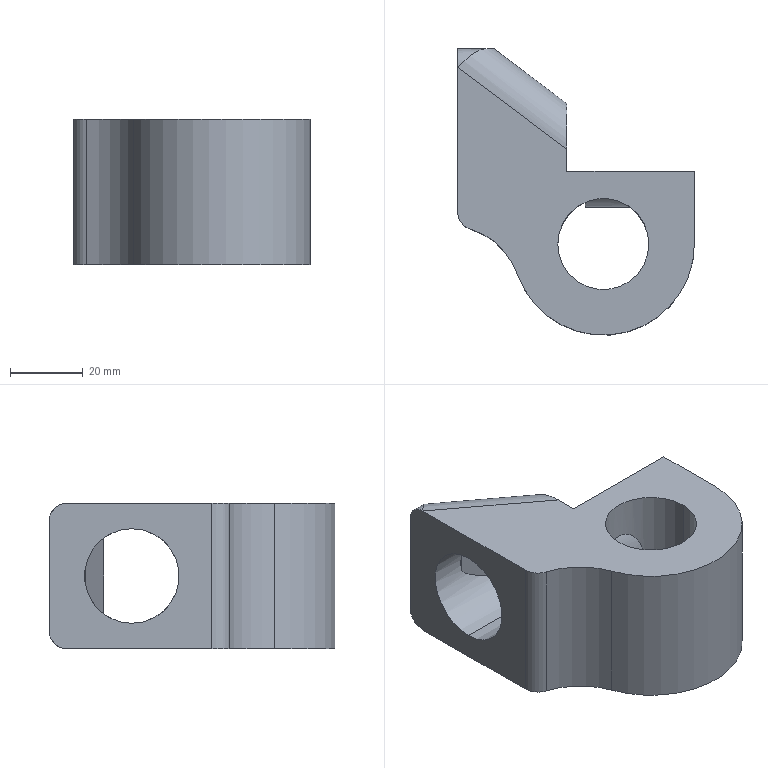Part | SolidWorks | features Cut 5, Fillet 4, ICE 4, Extrusion 1 | 1 solid | 29 faces | box 65 x 78.563 x 40 mm | volume 84441 mm3 | plane 15 | cylinder 14 | commonest cylinder face diameters 10 x3 41.45 x3 20 x2 25 x2 26 x2 40 x1
STEP:
#1=CARTESIAN_POINT('',(82.5,25.,40.));
#2=VERTEX_POINT('',#1);
#3=CARTESIAN_POINT('',(57.5,25.,40.));
#4=VERTEX_POINT('',#3);
#5=CARTESIAN_POINT('',(70.,25.,40.));
#6=DIRECTION('',(0.,0.,-1.));
#7=DIRECTION('',(-1.,0.,0.));
#8=AXIS2_PLACEMENT_3D('',#5,#6,#7);
#9=CIRCLE('',#8,12.5);
#10=EDGE_CURVE('',#2,#4,#9,.T.);
#11=ORIENTED_EDGE('',*,*,#10,.F.);
#12=CARTESIAN_POINT('',(82.5,25.,0.));
#13=VERTEX_POINT('',#12);
#14=CARTESIAN_POINT('',(82.5,25.,40.));
#15=DIRECTION('',(0.,0.,-1.));
#16=VECTOR('',#15,1000.);
#17=LINE('',#14,#16);
#18=EDGE_CURVE('',#2,#13,#17,.T.);
#19=ORIENTED_EDGE('',*,*,#18,.T.);
#20=CARTESIAN_POINT('',(57.5,25.,0.));
#21=VERTEX_POINT('',#20);
#22=CARTESIAN_POINT('',(70.,25.,0.));
#23=DIRECTION('',(0.,0.,1.));
#24=DIRECTION('',(1.,0.,0.));
#25=AXIS2_PLACEMENT_3D('',#22,#23,#24);
#26=CIRCLE('',#25,12.5);
#27=EDGE_CURVE('',#21,#13,#26,.T.);
#28=ORIENTED_EDGE('',*,*,#27,.F.);
#29=CARTESIAN_POINT('',(57.5,25.,40.));
#30=DIRECTION('',(0.,0.,-1.));
#31=VECTOR('',#30,1000.);
#32=LINE('',#29,#31);
#33=EDGE_CURVE('',#4,#21,#32,.T.);
#34=ORIENTED_EDGE('',*,*,#33,.F.);
#35=EDGE_LOOP('',(#11,#19,#28,#34));
#36=FACE_OUTER_BOUND('',#35,.T.);
#37=CARTESIAN_POINT('',(70.,25.,40.));
#38=DIRECTION('',(0.,0.,-1.));
#39=DIRECTION('',(-1.,0.,0.));
#40=AXIS2_PLACEMENT_3D('',#37,#38,#39);
#41=CYLINDRICAL_SURFACE('',#40,12.5);
#42=ADVANCED_FACE('',(#36),#41,.F.);
#43=CARTESIAN_POINT('',(60.,45.,12.81));
#44=VERTEX_POINT('',#43);
#45=CARTESIAN_POINT('',(60.,55.831,7.));
#46=VERTEX_POINT('',#45);
#47=CARTESIAN_POINT('',(60.,55.831,20.));
#48=DIRECTION('',(1.,0.,0.));
#49=DIRECTION('',(0.,0.,-1.));
#50=AXIS2_PLACEMENT_3D('',#47,#48,#49);
#51=CIRCLE('',#50,13.);
#52=EDGE_CURVE('',#44,#46,#51,.T.);
#53=ORIENTED_EDGE('',*,*,#52,.T.);
#54=CARTESIAN_POINT('',(30.,55.831,7.));
#55=VERTEX_POINT('',#54);
#56=CARTESIAN_POINT('',(95.,55.831,7.));
#57=DIRECTION('',(-1.,0.,0.));
#58=VECTOR('',#57,1000.);
#59=LINE('',#56,#58);
#60=EDGE_CURVE('',#46,#55,#59,.T.);
#61=ORIENTED_EDGE('',*,*,#60,.T.);
#62=CARTESIAN_POINT('',(30.,55.831,33.));
#63=VERTEX_POINT('',#62);
#64=CARTESIAN_POINT('',(30.,55.831,20.));
#65=DIRECTION('',(-1.,0.,0.));
#66=DIRECTION('',(0.,0.,1.));
#67=AXIS2_PLACEMENT_3D('',#64,#65,#66);
#68=CIRCLE('',#67,13.);
#69=EDGE_CURVE('',#55,#63,#68,.T.);
#70=ORIENTED_EDGE('',*,*,#69,.T.);
#71=CARTESIAN_POINT('',(60.,55.831,33.));
#72=VERTEX_POINT('',#71);
#73=CARTESIAN_POINT('',(95.,55.831,33.));
#74=DIRECTION('',(-1.,0.,0.));
#75=VECTOR('',#74,1000.);
#76=LINE('',#73,#75);
#77=EDGE_CURVE('',#72,#63,#76,.T.);
#78=ORIENTED_EDGE('',*,*,#77,.F.);
#79=CARTESIAN_POINT('',(60.,45.,27.19));
#80=VERTEX_POINT('',#79);
#81=CARTESIAN_POINT('',(60.,55.831,20.));
#82=DIRECTION('',(1.,0.,0.));
#83=DIRECTION('',(0.,0.,-1.));
#84=AXIS2_PLACEMENT_3D('',#81,#82,#83);
#85=CIRCLE('',#84,13.);
#86=EDGE_CURVE('',#72,#80,#85,.T.);
#87=ORIENTED_EDGE('',*,*,#86,.T.);
#88=CARTESIAN_POINT('',(65.,45.,27.19));
#89=VERTEX_POINT('',#88);
#90=CARTESIAN_POINT('',(95.,45.,27.19));
#91=DIRECTION('',(-1.,0.,0.));
#92=VECTOR('',#91,1000.);
#93=LINE('',#90,#92);
#94=EDGE_CURVE('',#89,#80,#93,.T.);
#95=ORIENTED_EDGE('',*,*,#94,.F.);
#96=CARTESIAN_POINT('',(65.,45.,12.81));
#97=VERTEX_POINT('',#96);
#98=CARTESIAN_POINT('',(65.,55.831,20.));
#99=DIRECTION('',(-1.,0.,0.));
#100=DIRECTION('',(0.,0.,-1.));
#101=AXIS2_PLACEMENT_3D('',#98,#99,#100);
#102=CIRCLE('',#101,13.);
#103=EDGE_CURVE('',#97,#89,#102,.T.);
#104=ORIENTED_EDGE('',*,*,#103,.F.);
#105=CARTESIAN_POINT('',(95.,45.,12.81));
#106=DIRECTION('',(1.,0.,0.));
#107=VECTOR('',#106,1000.);
#108=LINE('',#105,#107);
#109=EDGE_CURVE('',#44,#97,#108,.T.);
#110=ORIENTED_EDGE('',*,*,#109,.F.);
#111=EDGE_LOOP('',(#53,#61,#70,#78,#87,#95,#104,#110));
#112=FACE_OUTER_BOUND('',#111,.T.);
#113=CARTESIAN_POINT('',(95.,55.831,20.));
#114=DIRECTION('',(-1.,0.,0.));
#115=DIRECTION('',(0.,0.,1.));
#116=AXIS2_PLACEMENT_3D('',#113,#114,#115);
#117=CYLINDRICAL_SURFACE('',#116,13.);
#118=ADVANCED_FACE('',(#112),#117,.F.);
#119=CARTESIAN_POINT('',(95.,45.,37.67));
#120=VERTEX_POINT('',#119);
#121=CARTESIAN_POINT('',(95.,40.835,34.306));
#122=VERTEX_POINT('',#121);
#123=CARTESIAN_POINT('',(95.,55.831,20.));
#124=DIRECTION('',(1.,0.,0.));
#125=DIRECTION('',(0.,0.,-1.));
#126=AXIS2_PLACEMENT_3D('',#123,#124,#125);
#127=CIRCLE('',#126,20.725);
#128=EDGE_CURVE('',#120,#122,#127,.T.);
#129=ORIENTED_EDGE('',*,*,#128,.T.);
#130=CARTESIAN_POINT('',(65.,40.835,34.306));
#131=VERTEX_POINT('',#130);
#132=CARTESIAN_POINT('',(35.885,40.835,34.306));
#133=DIRECTION('',(1.,0.,0.));
#134=VECTOR('',#133,1000.);
#135=LINE('',#132,#134);
#136=EDGE_CURVE('',#131,#122,#135,.T.);
#137=ORIENTED_EDGE('',*,*,#136,.F.);
#138=CARTESIAN_POINT('',(65.,45.,37.67));
#139=VERTEX_POINT('',#138);
#140=CARTESIAN_POINT('',(65.,55.831,20.));
#141=DIRECTION('',(1.,0.,0.));
#142=DIRECTION('',(0.,0.,-1.));
#143=AXIS2_PLACEMENT_3D('',#140,#141,#142);
#144=CIRCLE('',#143,20.725);
#145=EDGE_CURVE('',#139,#131,#144,.T.);
#146=ORIENTED_EDGE('',*,*,#145,.F.);
#147=CARTESIAN_POINT('',(65.,45.,37.67));
#148=DIRECTION('',(1.,0.,0.));
#149=VECTOR('',#148,1000.);
#150=LINE('',#147,#149);
#151=EDGE_CURVE('',#139,#120,#150,.T.);
#152=ORIENTED_EDGE('',*,*,#151,.T.);
#153=EDGE_LOOP('',(#129,#137,#146,#152));
#154=FACE_OUTER_BOUND('',#153,.T.);
#155=CARTESIAN_POINT('',(65.,55.831,20.));
#156=DIRECTION('',(1.,0.,0.));
#157=DIRECTION('',(0.,0.,-1.));
#158=AXIS2_PLACEMENT_3D('',#155,#156,#157);
#159=CYLINDRICAL_SURFACE('',#158,20.725);
#160=ADVANCED_FACE('',(#154),#159,.F.);
#161=ORIENTED_EDGE('',*,*,#60,.F.);
#162=CARTESIAN_POINT('',(60.,63.55,9.54));
#163=VERTEX_POINT('',#162);
#164=CARTESIAN_POINT('',(60.,55.831,20.));
#165=DIRECTION('',(1.,0.,0.));
#166=DIRECTION('',(0.,0.,-1.));
#167=AXIS2_PLACEMENT_3D('',#164,#165,#166);
#168=CIRCLE('',#167,13.);
#169=EDGE_CURVE('',#46,#163,#168,.T.);
#170=ORIENTED_EDGE('',*,*,#169,.T.);
#171=CARTESIAN_POINT('',(59.975,63.569,9.554));
#172=VERTEX_POINT('',#171);
#173=CARTESIAN_POINT('',(60.,63.55,9.54));
#174=CARTESIAN_POINT('',(59.992,63.556,9.545));
#175=CARTESIAN_POINT('',(59.983,63.563,9.55));
#176=CARTESIAN_POINT('',(59.975,63.569,9.554));
#177=B_SPLINE_CURVE_WITH_KNOTS('',3,(#173,#174,#175,#176),.UNSPECIFIED.,.F.,.F.,(4,4),(0.,0.00003466),.UNSPECIFIED.);
#178=EDGE_CURVE('',#163,#172,#177,.T.);
#179=ORIENTED_EDGE('',*,*,#178,.T.);
#180=CARTESIAN_POINT('',(40.,68.563,17.377));
#181=VERTEX_POINT('',#180);
#182=CARTESIAN_POINT('',(59.975,63.569,9.554));
#183=CARTESIAN_POINT('',(49.576,66.169,11.481));
#184=CARTESIAN_POINT('',(42.611,67.91,14.208));
#185=CARTESIAN_POINT('',(40.,68.563,17.377));
#186=(BOUNDED_CURVE()B_SPLINE_CURVE(3,(#182,#183,#184,#185),.UNSPECIFIED.,.F.,.F.)B_SPLINE_CURVE_WITH_KNOTS((4,4),(5.35,6.08),.UNSPECIFIED.)CURVE()GEOMETRIC_REPRESENTATION_ITEM()RATIONAL_B_SPLINE_CURVE((1.,0.9561,0.9561,1.))REPRESENTATION_ITEM(''));
#187=EDGE_CURVE('',#172,#181,#186,.T.);
#188=ORIENTED_EDGE('',*,*,#187,.T.);
#189=CARTESIAN_POINT('',(40.,68.563,22.623));
#190=VERTEX_POINT('',#189);
#191=CARTESIAN_POINT('',(40.,55.831,20.));
#192=DIRECTION('',(1.,0.,0.));
#193=DIRECTION('',(0.,0.,-1.));
#194=AXIS2_PLACEMENT_3D('',#191,#192,#193);
#195=CIRCLE('',#194,13.);
#196=EDGE_CURVE('',#181,#190,#195,.T.);
#197=ORIENTED_EDGE('',*,*,#196,.T.);
#198=CARTESIAN_POINT('',(59.975,63.569,30.446));
#199=VERTEX_POINT('',#198);
#200=CARTESIAN_POINT('',(40.,68.563,22.623));
#201=CARTESIAN_POINT('',(42.611,67.91,25.792));
#202=CARTESIAN_POINT('',(49.576,66.169,28.519));
#203=CARTESIAN_POINT('',(59.975,63.569,30.446));
#204=(BOUNDED_CURVE()B_SPLINE_CURVE(3,(#200,#201,#202,#203),.UNSPECIFIED.,.F.,.T.)B_SPLINE_CURVE_WITH_KNOTS((4,4),(0.2032,0.9332),.UNSPECIFIED.)CURVE()GEOMETRIC_REPRESENTATION_ITEM()RATIONAL_B_SPLINE_CURVE((1.,0.9561,0.9561,1.))REPRESENTATION_ITEM(''));
#205=EDGE_CURVE('',#190,#199,#204,.T.);
#206=ORIENTED_EDGE('',*,*,#205,.T.);
#207=CARTESIAN_POINT('',(60.,63.55,30.46));
#208=VERTEX_POINT('',#207);
#209=CARTESIAN_POINT('',(59.975,63.569,30.446));
#210=CARTESIAN_POINT('',(59.983,63.563,30.45));
#211=CARTESIAN_POINT('',(59.992,63.556,30.455));
#212=CARTESIAN_POINT('',(60.,63.55,30.46));
#213=B_SPLINE_CURVE_WITH_KNOTS('',3,(#209,#210,#211,#212),.UNSPECIFIED.,.F.,.F.,(4,4),(0.,0.00003466),.UNSPECIFIED.);
#214=EDGE_CURVE('',#199,#208,#213,.T.);
#215=ORIENTED_EDGE('',*,*,#214,.T.);
#216=CARTESIAN_POINT('',(60.,55.831,20.));
#217=DIRECTION('',(1.,0.,0.));
#218=DIRECTION('',(0.,0.,-1.));
#219=AXIS2_PLACEMENT_3D('',#216,#217,#218);
#220=CIRCLE('',#219,13.);
#221=EDGE_CURVE('',#208,#72,#220,.T.);
#222=ORIENTED_EDGE('',*,*,#221,.T.);
#223=ORIENTED_EDGE('',*,*,#77,.T.);
#224=CARTESIAN_POINT('',(30.,55.831,20.));
#225=DIRECTION('',(-1.,0.,0.));
#226=DIRECTION('',(0.,0.,1.));
#227=AXIS2_PLACEMENT_3D('',#224,#225,#226);
#228=CIRCLE('',#227,13.);
#229=EDGE_CURVE('',#63,#55,#228,.T.);
#230=ORIENTED_EDGE('',*,*,#229,.T.);
#231=EDGE_LOOP('',(#161,#170,#179,#188,#197,#206,#215,#222,#223,#230));
#232=FACE_OUTER_BOUND('',#231,.T.);
#233=CARTESIAN_POINT('',(95.,55.831,20.));
#234=DIRECTION('',(-1.,0.,0.));
#235=DIRECTION('',(0.,0.,1.));
#236=AXIS2_PLACEMENT_3D('',#233,#234,#235);
#237=CYLINDRICAL_SURFACE('',#236,13.);
#238=ADVANCED_FACE('',(#232),#237,.F.);
#239=ORIENTED_EDGE('',*,*,#128,.F.);
#240=CARTESIAN_POINT('',(95.,45.,40.));
#241=VERTEX_POINT('',#240);
#242=CARTESIAN_POINT('',(95.,45.,0.));
#243=DIRECTION('',(0.,0.,-1.));
#244=VECTOR('',#243,1000.);
#245=LINE('',#242,#244);
#246=EDGE_CURVE('',#241,#120,#245,.T.);
#247=ORIENTED_EDGE('',*,*,#246,.F.);
#248=CARTESIAN_POINT('',(95.,25.,40.));
#249=VERTEX_POINT('',#248);
#250=CARTESIAN_POINT('',(95.,0.,40.));
#251=DIRECTION('',(0.,-1.,0.));
#252=VECTOR('',#251,1000.);
#253=LINE('',#250,#252);
#254=EDGE_CURVE('',#241,#249,#253,.T.);
#255=ORIENTED_EDGE('',*,*,#254,.T.);
#256=CARTESIAN_POINT('',(95.,25.,0.));
#257=VERTEX_POINT('',#256);
#258=CARTESIAN_POINT('',(95.,25.,40.));
#259=DIRECTION('',(0.,0.,-1.));
#260=VECTOR('',#259,1000.);
#261=LINE('',#258,#260);
#262=EDGE_CURVE('',#249,#257,#261,.T.);
#263=ORIENTED_EDGE('',*,*,#262,.T.);
#264=CARTESIAN_POINT('',(95.,45.,0.));
#265=VERTEX_POINT('',#264);
#266=CARTESIAN_POINT('',(95.,0.,0.));
#267=DIRECTION('',(0.,-1.,0.));
#268=VECTOR('',#267,1000.);
#269=LINE('',#266,#268);
#270=EDGE_CURVE('',#265,#257,#269,.T.);
#271=ORIENTED_EDGE('',*,*,#270,.F.);
#272=CARTESIAN_POINT('',(95.,45.,2.33));
#273=VERTEX_POINT('',#272);
#274=CARTESIAN_POINT('',(95.,45.,0.));
#275=DIRECTION('',(0.,0.,-1.));
#276=VECTOR('',#275,1000.);
#277=LINE('',#274,#276);
#278=EDGE_CURVE('',#273,#265,#277,.T.);
#279=ORIENTED_EDGE('',*,*,#278,.F.);
#280=CARTESIAN_POINT('',(95.,40.772,5.761));
#281=VERTEX_POINT('',#280);
#282=CARTESIAN_POINT('',(95.,55.831,20.));
#283=DIRECTION('',(1.,0.,0.));
#284=DIRECTION('',(0.,0.,-1.));
#285=AXIS2_PLACEMENT_3D('',#282,#283,#284);
#286=CIRCLE('',#285,20.725);
#287=EDGE_CURVE('',#281,#273,#286,.T.);
#288=ORIENTED_EDGE('',*,*,#287,.F.);
#289=CARTESIAN_POINT('',(95.,40.772,5.761));
#290=DIRECTION('',(0.,0.002218,1.));
#291=VECTOR('',#290,1000.);
#292=LINE('',#289,#291);
#293=EDGE_CURVE('',#281,#122,#292,.T.);
#294=ORIENTED_EDGE('',*,*,#293,.T.);
#295=EDGE_LOOP('',(#239,#247,#255,#263,#271,#279,#288,#294));
#296=FACE_OUTER_BOUND('',#295,.T.);
#297=CARTESIAN_POINT('',(95.,0.,40.));
#298=DIRECTION('',(1.,0.,0.));
#299=DIRECTION('',(0.,0.,-1.));
#300=AXIS2_PLACEMENT_3D('',#297,#298,#299);
#301=PLANE('',#300);
#302=ADVANCED_FACE('',(#296),#301,.T.);
#303=ORIENTED_EDGE('',*,*,#221,.F.);
#304=CARTESIAN_POINT('',(60.,51.063,40.));
#305=VERTEX_POINT('',#304);
#306=CARTESIAN_POINT('',(60.,63.55,30.46));
#307=CARTESIAN_POINT('',(60.,63.225,36.1));
#308=CARTESIAN_POINT('',(60.,58.121,40.));
#309=CARTESIAN_POINT('',(60.,51.063,40.));
#310=(BOUNDED_CURVE()B_SPLINE_CURVE(3,(#306,#307,#308,#309),.UNSPECIFIED.,.F.,.T.)B_SPLINE_CURVE_WITH_KNOTS((4,4),(3.188,4.712),.UNSPECIFIED.)CURVE()GEOMETRIC_REPRESENTATION_ITEM()RATIONAL_B_SPLINE_CURVE((1.,0.8155,0.8155,1.))REPRESENTATION_ITEM(''));
#311=EDGE_CURVE('',#208,#305,#310,.T.);
#312=ORIENTED_EDGE('',*,*,#311,.T.);
#313=CARTESIAN_POINT('',(60.,45.,40.));
#314=VERTEX_POINT('',#313);
#315=CARTESIAN_POINT('',(60.,29.867,40.));
#316=DIRECTION('',(0.,-1.,0.));
#317=VECTOR('',#316,1000.);
#318=LINE('',#315,#317);
#319=EDGE_CURVE('',#305,#314,#318,.T.);
#320=ORIENTED_EDGE('',*,*,#319,.T.);
#321=CARTESIAN_POINT('',(60.,45.,0.));
#322=DIRECTION('',(0.,0.,1.));
#323=VECTOR('',#322,1000.);
#324=LINE('',#321,#323);
#325=EDGE_CURVE('',#80,#314,#324,.T.);
#326=ORIENTED_EDGE('',*,*,#325,.F.);
#327=ORIENTED_EDGE('',*,*,#86,.F.);
#328=EDGE_LOOP('',(#303,#312,#320,#326,#327));
#329=FACE_OUTER_BOUND('',#328,.T.);
#330=CARTESIAN_POINT('',(60.,0.,0.));
#331=DIRECTION('',(1.,0.,0.));
#332=DIRECTION('',(0.,0.,-1.));
#333=AXIS2_PLACEMENT_3D('',#330,#331,#332);
#334=PLANE('',#333);
#335=ADVANCED_FACE('',(#329),#334,.T.);
#336=CARTESIAN_POINT('',(60.,45.,0.));
#337=VERTEX_POINT('',#336);
#338=CARTESIAN_POINT('',(60.,51.063,0.));
#339=VERTEX_POINT('',#338);
#340=CARTESIAN_POINT('',(60.,29.867,0.));
#341=DIRECTION('',(0.,1.,0.));
#342=VECTOR('',#341,1000.);
#343=LINE('',#340,#342);
#344=EDGE_CURVE('',#337,#339,#343,.T.);
#345=ORIENTED_EDGE('',*,*,#344,.T.);
#346=CARTESIAN_POINT('',(60.,51.063,0.));
#347=CARTESIAN_POINT('',(60.,58.121,0.));
#348=CARTESIAN_POINT('',(60.,63.225,3.9));
#349=CARTESIAN_POINT('',(60.,63.55,9.54));
#350=(BOUNDED_CURVE()B_SPLINE_CURVE(3,(#346,#347,#348,#349),.UNSPECIFIED.,.F.,.F.)B_SPLINE_CURVE_WITH_KNOTS((4,4),(4.712,6.237),.UNSPECIFIED.)CURVE()GEOMETRIC_REPRESENTATION_ITEM()RATIONAL_B_SPLINE_CURVE((1.,0.8155,0.8155,1.))REPRESENTATION_ITEM(''));
#351=EDGE_CURVE('',#339,#163,#350,.T.);
#352=ORIENTED_EDGE('',*,*,#351,.T.);
#353=ORIENTED_EDGE('',*,*,#169,.F.);
#354=ORIENTED_EDGE('',*,*,#52,.F.);
#355=CARTESIAN_POINT('',(60.,45.,0.));
#356=DIRECTION('',(0.,0.,1.));
#357=VECTOR('',#356,1000.);
#358=LINE('',#355,#357);
#359=EDGE_CURVE('',#337,#44,#358,.T.);
#360=ORIENTED_EDGE('',*,*,#359,.F.);
#361=EDGE_LOOP('',(#345,#352,#353,#354,#360));
#362=FACE_OUTER_BOUND('',#361,.T.);
#363=CARTESIAN_POINT('',(60.,0.,0.));
#364=DIRECTION('',(1.,0.,0.));
#365=DIRECTION('',(0.,0.,-1.));
#366=AXIS2_PLACEMENT_3D('',#363,#364,#365);
#367=PLANE('',#366);
#368=ADVANCED_FACE('',(#362),#367,.T.);
#369=ORIENTED_EDGE('',*,*,#262,.F.);
#370=CARTESIAN_POINT('',(46.427,16.675,40.));
#371=VERTEX_POINT('',#370);
#372=CARTESIAN_POINT('',(70.,25.,40.));
#373=DIRECTION('',(0.,0.,1.));
#374=DIRECTION('',(1.,0.,0.));
#375=AXIS2_PLACEMENT_3D('',#372,#373,#374);
#376=CIRCLE('',#375,25.);
#377=EDGE_CURVE('',#371,#249,#376,.T.);
#378=ORIENTED_EDGE('',*,*,#377,.F.);
#379=CARTESIAN_POINT('',(46.427,16.675,0.));
#380=VERTEX_POINT('',#379);
#381=CARTESIAN_POINT('',(46.427,16.675,40.));
#382=DIRECTION('',(0.,0.,-1.));
#383=VECTOR('',#382,1000.);
#384=LINE('',#381,#383);
#385=EDGE_CURVE('',#371,#380,#384,.T.);
#386=ORIENTED_EDGE('',*,*,#385,.T.);
#387=CARTESIAN_POINT('',(70.,25.,0.));
#388=DIRECTION('',(0.,0.,1.));
#389=DIRECTION('',(1.,0.,0.));
#390=AXIS2_PLACEMENT_3D('',#387,#388,#389);
#391=CIRCLE('',#390,25.);
#392=EDGE_CURVE('',#380,#257,#391,.T.);
#393=ORIENTED_EDGE('',*,*,#392,.T.);
#394=EDGE_LOOP('',(#369,#378,#386,#393));
#395=FACE_OUTER_BOUND('',#394,.T.);
#396=CARTESIAN_POINT('',(70.,25.,40.));
#397=DIRECTION('',(0.,0.,-1.));
#398=DIRECTION('',(-1.,0.,0.));
#399=AXIS2_PLACEMENT_3D('',#396,#397,#398);
#400=CYLINDRICAL_SURFACE('',#399,25.);
#401=ADVANCED_FACE('',(#395),#400,.T.);
#402=ORIENTED_EDGE('',*,*,#319,.F.);
#403=CARTESIAN_POINT('',(30.,73.563,40.));
#404=VERTEX_POINT('',#403);
#405=CARTESIAN_POINT('',(78.91,36.88,40.));
#406=DIRECTION('',(-0.8,0.6,0.));
#407=VECTOR('',#406,1000.);
#408=LINE('',#405,#407);
#409=EDGE_CURVE('',#305,#404,#408,.T.);
#410=ORIENTED_EDGE('',*,*,#409,.T.);
#411=CARTESIAN_POINT('',(30.,33.885,40.));
#412=VERTEX_POINT('',#411);
#413=CARTESIAN_POINT('',(30.,29.867,40.));
#414=DIRECTION('',(0.,-1.,0.));
#415=VECTOR('',#414,1000.);
#416=LINE('',#413,#415);
#417=EDGE_CURVE('',#404,#412,#416,.T.);
#418=ORIENTED_EDGE('',*,*,#417,.T.);
#419=CARTESIAN_POINT('',(33.514,29.112,40.));
#420=VERTEX_POINT('',#419);
#421=CARTESIAN_POINT('',(35.,33.885,40.));
#422=DIRECTION('',(0.,0.,1.));
#423=DIRECTION('',(1.,0.,0.));
#424=AXIS2_PLACEMENT_3D('',#421,#422,#423);
#425=CIRCLE('',#424,5.);
#426=EDGE_CURVE('',#412,#420,#425,.T.);
#427=ORIENTED_EDGE('',*,*,#426,.T.);
#428=CARTESIAN_POINT('',(27.568,10.016,40.));
#429=DIRECTION('',(0.,0.,-1.));
#430=DIRECTION('',(1.,0.,0.));
#431=AXIS2_PLACEMENT_3D('',#428,#429,#430);
#432=CIRCLE('',#431,20.);
#433=EDGE_CURVE('',#420,#371,#432,.T.);
#434=ORIENTED_EDGE('',*,*,#433,.T.);
#435=ORIENTED_EDGE('',*,*,#377,.T.);
#436=ORIENTED_EDGE('',*,*,#254,.F.);
#437=CARTESIAN_POINT('',(60.,45.,40.));
#438=DIRECTION('',(1.,0.,0.));
#439=VECTOR('',#438,1000.);
#440=LINE('',#437,#439);
#441=EDGE_CURVE('',#314,#241,#440,.T.);
#442=ORIENTED_EDGE('',*,*,#441,.F.);
#443=EDGE_LOOP('',(#402,#410,#418,#427,#434,#435,#436,#442));
#444=FACE_OUTER_BOUND('',#443,.T.);
#445=CARTESIAN_POINT('',(70.,25.,40.));
#446=DIRECTION('',(0.,0.,-1.));
#447=DIRECTION('',(-1.,0.,0.));
#448=AXIS2_PLACEMENT_3D('',#445,#446,#447);
#449=CIRCLE('',#448,12.5);
#450=EDGE_CURVE('',#4,#2,#449,.T.);
#451=ORIENTED_EDGE('',*,*,#450,.T.);
#452=ORIENTED_EDGE('',*,*,#10,.T.);
#453=EDGE_LOOP('',(#451,#452));
#454=FACE_BOUND('',#453,.T.);
#455=CARTESIAN_POINT('',(70.,25.,40.));
#456=DIRECTION('',(0.,0.,1.));
#457=DIRECTION('',(1.,0.,0.));
#458=AXIS2_PLACEMENT_3D('',#455,#456,#457);
#459=PLANE('',#458);
#460=ADVANCED_FACE('',(#444,#454),#459,.T.);
#461=ORIENTED_EDGE('',*,*,#27,.T.);
#462=CARTESIAN_POINT('',(70.,25.,0.));
#463=DIRECTION('',(0.,0.,1.));
#464=DIRECTION('',(1.,0.,0.));
#465=AXIS2_PLACEMENT_3D('',#462,#463,#464);
#466=CIRCLE('',#465,12.5);
#467=EDGE_CURVE('',#13,#21,#466,.T.);
#468=ORIENTED_EDGE('',*,*,#467,.T.);
#469=EDGE_LOOP('',(#461,#468));
#470=FACE_BOUND('',#469,.T.);
#471=CARTESIAN_POINT('',(30.,33.885,0.));
#472=VERTEX_POINT('',#471);
#473=CARTESIAN_POINT('',(30.,73.563,0.));
#474=VERTEX_POINT('',#473);
#475=CARTESIAN_POINT('',(30.,29.867,0.));
#476=DIRECTION('',(0.,1.,0.));
#477=VECTOR('',#476,1000.);
#478=LINE('',#475,#477);
#479=EDGE_CURVE('',#472,#474,#478,.T.);
#480=ORIENTED_EDGE('',*,*,#479,.T.);
#481=CARTESIAN_POINT('',(54.,55.563,0.));
#482=DIRECTION('',(0.8,-0.6,0.));
#483=VECTOR('',#482,1000.);
#484=LINE('',#481,#483);
#485=EDGE_CURVE('',#474,#339,#484,.T.);
#486=ORIENTED_EDGE('',*,*,#485,.T.);
#487=ORIENTED_EDGE('',*,*,#344,.F.);
#488=CARTESIAN_POINT('',(60.,45.,0.));
#489=DIRECTION('',(-1.,0.,0.));
#490=VECTOR('',#489,1000.);
#491=LINE('',#488,#490);
#492=EDGE_CURVE('',#265,#337,#491,.T.);
#493=ORIENTED_EDGE('',*,*,#492,.F.);
#494=ORIENTED_EDGE('',*,*,#270,.T.);
#495=ORIENTED_EDGE('',*,*,#392,.F.);
#496=CARTESIAN_POINT('',(33.514,29.112,0.));
#497=VERTEX_POINT('',#496);
#498=CARTESIAN_POINT('',(27.568,10.016,0.));
#499=DIRECTION('',(0.,0.,1.));
#500=DIRECTION('',(1.,0.,0.));
#501=AXIS2_PLACEMENT_3D('',#498,#499,#500);
#502=CIRCLE('',#501,20.);
#503=EDGE_CURVE('',#380,#497,#502,.T.);
#504=ORIENTED_EDGE('',*,*,#503,.T.);
#505=CARTESIAN_POINT('',(35.,33.885,0.));
#506=DIRECTION('',(0.,0.,-1.));
#507=DIRECTION('',(1.,0.,0.));
#508=AXIS2_PLACEMENT_3D('',#505,#506,#507);
#509=CIRCLE('',#508,5.);
#510=EDGE_CURVE('',#497,#472,#509,.T.);
#511=ORIENTED_EDGE('',*,*,#510,.T.);
#512=EDGE_LOOP('',(#480,#486,#487,#493,#494,#495,#504,#511));
#513=FACE_OUTER_BOUND('',#512,.T.);
#514=CARTESIAN_POINT('',(70.,25.,0.));
#515=DIRECTION('',(0.,0.,1.));
#516=DIRECTION('',(1.,0.,0.));
#517=AXIS2_PLACEMENT_3D('',#514,#515,#516);
#518=PLANE('',#517);
#519=ADVANCED_FACE('',(#470,#513),#518,.F.);
#520=CARTESIAN_POINT('',(30.,78.563,35.));
#521=VERTEX_POINT('',#520);
#522=CARTESIAN_POINT('',(37.767,78.563,35.));
#523=VERTEX_POINT('',#522);
#524=CARTESIAN_POINT('',(30.,78.563,35.));
#525=DIRECTION('',(1.,0.,0.));
#526=VECTOR('',#525,1000.);
#527=LINE('',#524,#526);
#528=EDGE_CURVE('',#521,#523,#527,.T.);
#529=ORIENTED_EDGE('',*,*,#528,.T.);
#530=CARTESIAN_POINT('',(40.,78.563,30.));
#531=VERTEX_POINT('',#530);
#532=CARTESIAN_POINT('',(37.767,78.563,35.));
#533=CARTESIAN_POINT('',(39.238,78.563,33.471));
#534=CARTESIAN_POINT('',(40.,78.563,31.766));
#535=CARTESIAN_POINT('',(40.,78.563,30.));
#536=(BOUNDED_CURVE()B_SPLINE_CURVE(3,(#532,#533,#534,#535),.UNSPECIFIED.,.F.,.F.)B_SPLINE_CURVE_WITH_KNOTS((4,4),(5.76,6.283),.UNSPECIFIED.)CURVE()GEOMETRIC_REPRESENTATION_ITEM()RATIONAL_B_SPLINE_CURVE((1.,0.9773,0.9773,1.))REPRESENTATION_ITEM(''));
#537=EDGE_CURVE('',#523,#531,#536,.T.);
#538=ORIENTED_EDGE('',*,*,#537,.T.);
#539=CARTESIAN_POINT('',(40.,78.563,10.));
#540=VERTEX_POINT('',#539);
#541=CARTESIAN_POINT('',(40.,78.563,40.));
#542=DIRECTION('',(0.,0.,-1.));
#543=VECTOR('',#542,1000.);
#544=LINE('',#541,#543);
#545=EDGE_CURVE('',#531,#540,#544,.T.);
#546=ORIENTED_EDGE('',*,*,#545,.T.);
#547=CARTESIAN_POINT('',(37.767,78.563,5.));
#548=VERTEX_POINT('',#547);
#549=CARTESIAN_POINT('',(40.,78.563,10.));
#550=CARTESIAN_POINT('',(40.,78.563,8.234));
#551=CARTESIAN_POINT('',(39.238,78.563,6.529));
#552=CARTESIAN_POINT('',(37.767,78.563,5.));
#553=(BOUNDED_CURVE()B_SPLINE_CURVE(3,(#549,#550,#551,#552),.UNSPECIFIED.,.F.,.F.)B_SPLINE_CURVE_WITH_KNOTS((4,4),(3.142,3.665),.UNSPECIFIED.)CURVE()GEOMETRIC_REPRESENTATION_ITEM()RATIONAL_B_SPLINE_CURVE((1.,0.9773,0.9773,1.))REPRESENTATION_ITEM(''));
#554=EDGE_CURVE('',#540,#548,#553,.T.);
#555=ORIENTED_EDGE('',*,*,#554,.T.);
#556=CARTESIAN_POINT('',(30.,78.563,5.));
#557=VERTEX_POINT('',#556);
#558=CARTESIAN_POINT('',(30.,78.563,5.));
#559=DIRECTION('',(-1.,0.,0.));
#560=VECTOR('',#559,1000.);
#561=LINE('',#558,#560);
#562=EDGE_CURVE('',#548,#557,#561,.T.);
#563=ORIENTED_EDGE('',*,*,#562,.T.);
#564=CARTESIAN_POINT('',(30.,78.563,0.));
#565=DIRECTION('',(0.,0.,1.));
#566=VECTOR('',#565,1000.);
#567=LINE('',#564,#566);
#568=EDGE_CURVE('',#557,#521,#567,.T.);
#569=ORIENTED_EDGE('',*,*,#568,.T.);
#570=EDGE_LOOP('',(#529,#538,#546,#555,#563,#569));
#571=FACE_OUTER_BOUND('',#570,.T.);
#572=CARTESIAN_POINT('',(30.,78.563,0.));
#573=DIRECTION('',(0.,1.,0.));
#574=DIRECTION('',(0.,0.,1.));
#575=AXIS2_PLACEMENT_3D('',#572,#573,#574);
#576=PLANE('',#575);
#577=ADVANCED_FACE('',(#571),#576,.T.);
#578=ORIENTED_EDGE('',*,*,#229,.F.);
#579=ORIENTED_EDGE('',*,*,#69,.F.);
#580=EDGE_LOOP('',(#578,#579));
#581=FACE_BOUND('',#580,.T.);
#582=ORIENTED_EDGE('',*,*,#479,.F.);
#583=CARTESIAN_POINT('',(30.,33.885,0.));
#584=DIRECTION('',(0.,0.,1.));
#585=VECTOR('',#584,1000.);
#586=LINE('',#583,#585);
#587=EDGE_CURVE('',#472,#412,#586,.T.);
#588=ORIENTED_EDGE('',*,*,#587,.T.);
#589=ORIENTED_EDGE('',*,*,#417,.F.);
#590=CARTESIAN_POINT('',(30.,73.563,35.));
#591=DIRECTION('',(-1.,0.,0.));
#592=DIRECTION('',(0.,0.,-1.));
#593=AXIS2_PLACEMENT_3D('',#590,#591,#592);
#594=CIRCLE('',#593,5.);
#595=EDGE_CURVE('',#404,#521,#594,.T.);
#596=ORIENTED_EDGE('',*,*,#595,.T.);
#597=ORIENTED_EDGE('',*,*,#568,.F.);
#598=CARTESIAN_POINT('',(30.,73.563,5.));
#599=DIRECTION('',(-1.,0.,0.));
#600=DIRECTION('',(0.,0.,-1.));
#601=AXIS2_PLACEMENT_3D('',#598,#599,#600);
#602=CIRCLE('',#601,5.);
#603=EDGE_CURVE('',#557,#474,#602,.T.);
#604=ORIENTED_EDGE('',*,*,#603,.T.);
#605=EDGE_LOOP('',(#582,#588,#589,#596,#597,#604));
#606=FACE_OUTER_BOUND('',#605,.T.);
#607=CARTESIAN_POINT('',(30.,0.,0.));
#608=DIRECTION('',(1.,0.,0.));
#609=DIRECTION('',(0.,0.,-1.));
#610=AXIS2_PLACEMENT_3D('',#607,#608,#609);
#611=PLANE('',#610);
#612=ADVANCED_FACE('',(#581,#606),#611,.F.);
#613=ORIENTED_EDGE('',*,*,#595,.F.);
#614=CARTESIAN_POINT('',(30.,73.563,40.));
#615=CARTESIAN_POINT('',(30.331,73.887,40.));
#616=CARTESIAN_POINT('',(30.663,74.211,39.968));
#617=CARTESIAN_POINT('',(31.325,74.847,39.843));
#618=CARTESIAN_POINT('',(31.652,75.156,39.751));
#619=CARTESIAN_POINT('',(32.304,75.751,39.507));
#620=CARTESIAN_POINT('',(32.629,76.038,39.357));
#621=CARTESIAN_POINT('',(33.282,76.582,38.999));
#622=CARTESIAN_POINT('',(33.61,76.839,38.791));
#623=CARTESIAN_POINT('',(34.255,77.304,38.333));
#624=CARTESIAN_POINT('',(34.574,77.514,38.082));
#625=CARTESIAN_POINT('',(35.215,77.884,37.538));
#626=CARTESIAN_POINT('',(35.539,78.044,37.243));
#627=CARTESIAN_POINT('',(36.498,78.43,36.325));
#628=CARTESIAN_POINT('',(37.123,78.563,35.669));
#629=CARTESIAN_POINT('',(37.767,78.563,35.));
#630=B_SPLINE_CURVE_WITH_KNOTS('',3,(#614,#615,#616,#617,#618,#619,#620,#621,#622,#623,#624,#625,#626,#627,#628,#629),.UNSPECIFIED.,.F.,.F.,(4,2,2,2,2,2,2,4),(-0.00002872,0.001361,0.00275,0.00414,0.00553,0.006919,0.008309,0.01109),.UNSPECIFIED.);
#631=EDGE_CURVE('',#404,#523,#630,.T.);
#632=ORIENTED_EDGE('',*,*,#631,.T.);
#633=ORIENTED_EDGE('',*,*,#528,.F.);
#634=EDGE_LOOP('',(#613,#632,#633));
#635=FACE_OUTER_BOUND('',#634,.T.);
#636=CARTESIAN_POINT('',(30.,73.563,35.));
#637=DIRECTION('',(1.,0.,0.));
#638=DIRECTION('',(0.,0.,-1.));
#639=AXIS2_PLACEMENT_3D('',#636,#637,#638);
#640=CYLINDRICAL_SURFACE('',#639,5.);
#641=ADVANCED_FACE('',(#635),#640,.T.);
#642=ORIENTED_EDGE('',*,*,#562,.F.);
#643=CARTESIAN_POINT('',(37.767,78.563,5.));
#644=CARTESIAN_POINT('',(37.123,78.563,4.331));
#645=CARTESIAN_POINT('',(36.498,78.43,3.675));
#646=CARTESIAN_POINT('',(35.539,78.044,2.757));
#647=CARTESIAN_POINT('',(35.215,77.884,2.462));
#648=CARTESIAN_POINT('',(34.574,77.514,1.918));
#649=CARTESIAN_POINT('',(34.254,77.304,1.667));
#650=CARTESIAN_POINT('',(33.609,76.839,1.209));
#651=CARTESIAN_POINT('',(33.282,76.582,1.001));
#652=CARTESIAN_POINT('',(32.628,76.037,0.6429));
#653=CARTESIAN_POINT('',(32.303,75.751,0.4926));
#654=CARTESIAN_POINT('',(31.652,75.155,0.2494));
#655=CARTESIAN_POINT('',(31.325,74.847,0.1567));
#656=CARTESIAN_POINT('',(30.829,74.37,0.06286));
#657=CARTESIAN_POINT('',(30.663,74.209,0.03926));
#658=CARTESIAN_POINT('',(30.414,73.967,0.01571));
#659=CARTESIAN_POINT('',(30.331,73.887,0.00982));
#660=CARTESIAN_POINT('',(30.166,73.725,0.001962));
#661=CARTESIAN_POINT('',(30.082,73.643,0.));
#662=CARTESIAN_POINT('',(30.,73.563,0.));
#663=B_SPLINE_CURVE_WITH_KNOTS('',3,(#643,#644,#645,#646,#647,#648,#649,#650,#651,#652,#653,#654,#655,#656,#657,#658,#659,#660,#661,#662),.UNSPECIFIED.,.F.,.F.,(4,2,2,2,2,2,2,2,2,4),(0.,0.002746,0.004119,0.005492,0.006865,0.008238,0.009611,0.0103,0.01064,0.01098),.UNSPECIFIED.);
#664=EDGE_CURVE('',#548,#474,#663,.T.);
#665=ORIENTED_EDGE('',*,*,#664,.T.);
#666=ORIENTED_EDGE('',*,*,#603,.F.);
#667=EDGE_LOOP('',(#642,#665,#666));
#668=FACE_OUTER_BOUND('',#667,.T.);
#669=CARTESIAN_POINT('',(70.,73.563,5.));
#670=DIRECTION('',(-1.,0.,0.));
#671=DIRECTION('',(0.,0.,1.));
#672=AXIS2_PLACEMENT_3D('',#669,#670,#671);
#673=CYLINDRICAL_SURFACE('',#672,5.);
#674=ADVANCED_FACE('',(#668),#673,.T.);
#675=ORIENTED_EDGE('',*,*,#433,.F.);
#676=CARTESIAN_POINT('',(33.514,29.112,0.));
#677=DIRECTION('',(0.,0.,-1.));
#678=VECTOR('',#677,1000.);
#679=LINE('',#676,#678);
#680=EDGE_CURVE('',#420,#497,#679,.T.);
#681=ORIENTED_EDGE('',*,*,#680,.T.);
#682=ORIENTED_EDGE('',*,*,#503,.F.);
#683=ORIENTED_EDGE('',*,*,#385,.F.);
#684=EDGE_LOOP('',(#675,#681,#682,#683));
#685=FACE_OUTER_BOUND('',#684,.T.);
#686=CARTESIAN_POINT('',(27.568,10.016,0.));
#687=DIRECTION('',(0.,0.,1.));
#688=DIRECTION('',(1.,0.,0.));
#689=AXIS2_PLACEMENT_3D('',#686,#687,#688);
#690=CYLINDRICAL_SURFACE('',#689,20.);
#691=ADVANCED_FACE('',(#685),#690,.F.);
#692=ORIENTED_EDGE('',*,*,#426,.F.);
#693=ORIENTED_EDGE('',*,*,#587,.F.);
#694=ORIENTED_EDGE('',*,*,#510,.F.);
#695=ORIENTED_EDGE('',*,*,#680,.F.);
#696=EDGE_LOOP('',(#692,#693,#694,#695));
#697=FACE_OUTER_BOUND('',#696,.T.);
#698=CARTESIAN_POINT('',(35.,33.885,0.));
#699=DIRECTION('',(0.,0.,1.));
#700=DIRECTION('',(1.,0.,0.));
#701=AXIS2_PLACEMENT_3D('',#698,#699,#700);
#702=CYLINDRICAL_SURFACE('',#701,5.);
#703=ADVANCED_FACE('',(#697),#702,.T.);
#704=ORIENTED_EDGE('',*,*,#18,.F.);
#705=ORIENTED_EDGE('',*,*,#450,.F.);
#706=ORIENTED_EDGE('',*,*,#33,.T.);
#707=ORIENTED_EDGE('',*,*,#467,.F.);
#708=EDGE_LOOP('',(#704,#705,#706,#707));
#709=FACE_OUTER_BOUND('',#708,.T.);
#710=CARTESIAN_POINT('',(65.,36.456,27.36));
#711=VERTEX_POINT('',#710);
#712=CARTESIAN_POINT('',(65.,36.456,12.64));
#713=VERTEX_POINT('',#712);
#714=CARTESIAN_POINT('',(65.,36.456,40.));
#715=DIRECTION('',(0.,0.,-1.));
#716=VECTOR('',#715,1000.);
#717=LINE('',#714,#716);
#718=EDGE_CURVE('',#711,#713,#717,.T.);
#719=ORIENTED_EDGE('',*,*,#718,.F.);
#720=CARTESIAN_POINT('',(65.,36.456,27.36));
#721=CARTESIAN_POINT('',(65.26,36.57,27.659));
#722=CARTESIAN_POINT('',(65.542,36.682,27.933));
#723=CARTESIAN_POINT('',(65.998,36.843,28.308));
#724=CARTESIAN_POINT('',(66.156,36.896,28.426));
#725=CARTESIAN_POINT('',(66.485,36.997,28.65));
#726=CARTESIAN_POINT('',(66.656,37.046,28.756));
#727=CARTESIAN_POINT('',(67.181,37.183,29.047));
#728=CARTESIAN_POINT('',(67.546,37.263,29.208));
#729=CARTESIAN_POINT('',(68.31,37.391,29.462));
#730=CARTESIAN_POINT('',(68.713,37.44,29.556));
#731=CARTESIAN_POINT('',(69.52,37.497,29.665));
#732=CARTESIAN_POINT('',(69.927,37.506,29.682));
#733=CARTESIAN_POINT('',(70.54,37.49,29.651));
#734=CARTESIAN_POINT('',(70.747,37.479,29.631));
#735=CARTESIAN_POINT('',(71.152,37.448,29.572));
#736=CARTESIAN_POINT('',(71.352,37.428,29.533));
#737=CARTESIAN_POINT('',(71.942,37.355,29.39));
#738=CARTESIAN_POINT('',(72.326,37.287,29.258));
#739=CARTESIAN_POINT('',(73.062,37.125,28.925));
#740=CARTESIAN_POINT('',(73.407,37.032,28.728));
#741=CARTESIAN_POINT('',(74.057,36.828,28.276));
#742=CARTESIAN_POINT('',(74.364,36.717,28.019));
#743=CARTESIAN_POINT('',(74.922,36.494,27.464));
#744=CARTESIAN_POINT('',(75.177,36.381,27.165));
#745=CARTESIAN_POINT('',(75.641,36.158,26.528));
#746=CARTESIAN_POINT('',(75.852,36.048,26.188));
#747=CARTESIAN_POINT('',(76.223,35.843,25.492));
#748=CARTESIAN_POINT('',(76.385,35.747,25.132));
#749=CARTESIAN_POINT('',(76.671,35.573,24.391));
#750=CARTESIAN_POINT('',(76.794,35.493,24.01));
#751=CARTESIAN_POINT('',(77.003,35.355,23.228));
#752=CARTESIAN_POINT('',(77.089,35.296,22.832));
#753=CARTESIAN_POINT('',(77.224,35.202,22.034));
#754=CARTESIAN_POINT('',(77.274,35.166,21.631));
#755=CARTESIAN_POINT('',(77.34,35.118,20.82));
#756=CARTESIAN_POINT('',(77.357,35.106,20.41));
#757=CARTESIAN_POINT('',(77.357,35.106,19.18));
#758=CARTESIAN_POINT('',(77.292,35.154,18.372));
#759=CARTESIAN_POINT('',(77.091,35.295,17.179));
#760=CARTESIAN_POINT('',(77.006,35.353,16.785));
#761=CARTESIAN_POINT('',(76.797,35.491,16.002));
#762=CARTESIAN_POINT('',(76.674,35.57,15.619));
#763=CARTESIAN_POINT('',(76.389,35.745,14.877));
#764=CARTESIAN_POINT('',(76.227,35.841,14.517));
#765=CARTESIAN_POINT('',(75.857,36.045,13.82));
#766=CARTESIAN_POINT('',(75.647,36.155,13.481));
#767=CARTESIAN_POINT('',(75.183,36.378,12.843));
#768=CARTESIAN_POINT('',(74.93,36.491,12.545));
#769=CARTESIAN_POINT('',(74.513,36.658,12.129));
#770=CARTESIAN_POINT('',(74.369,36.713,11.997));
#771=CARTESIAN_POINT('',(74.066,36.821,11.742));
#772=CARTESIAN_POINT('',(73.907,36.875,11.62));
#773=CARTESIAN_POINT('',(73.418,37.029,11.278));
#774=CARTESIAN_POINT('',(73.073,37.122,11.081));
#775=CARTESIAN_POINT('',(72.345,37.284,10.749));
#776=CARTESIAN_POINT('',(71.956,37.352,10.614));
#777=CARTESIAN_POINT('',(71.168,37.452,10.421));
#778=CARTESIAN_POINT('',(70.767,37.483,10.362));
#779=CARTESIAN_POINT('',(70.154,37.501,10.328));
#780=CARTESIAN_POINT('',(69.947,37.502,10.327));
#781=CARTESIAN_POINT('',(69.535,37.493,10.343));
#782=CARTESIAN_POINT('',(69.331,37.484,10.361));
#783=CARTESIAN_POINT('',(68.726,37.441,10.441));
#784=CARTESIAN_POINT('',(68.329,37.394,10.532));
#785=CARTESIAN_POINT('',(67.554,37.265,10.789));
#786=CARTESIAN_POINT('',(67.187,37.185,10.95));
#787=CARTESIAN_POINT('',(66.489,37.002,11.336));
#788=CARTESIAN_POINT('',(66.157,36.899,11.563));
#789=CARTESIAN_POINT('',(65.543,36.683,12.065));
#790=CARTESIAN_POINT('',(65.261,36.57,12.341));
#791=CARTESIAN_POINT('',(65.,36.456,12.64));
#792=B_SPLINE_CURVE_WITH_KNOTS('',3,(#720,#721,#722,#723,#724,#725,#726,#727,#728,#729,#730,#731,#732,#733,#734,#735,#736,#737,#738,#739,#740,#741,#742,#743,#744,#745,#746,#747,#748,#749,#750,#751,#752,#753,#754,#755,#756,#757,#758,#759,#760,#761,#762,#763,#764,#765,#766,#767,#768,#769,#770,#771,#772,#773,#774,#775,#776,#777,#778,#779,#780,#781,#782,#783,#784,#785,#786,#787,#788,#789,#790,#791),.UNSPECIFIED.,.F.,.F.,(4,2,2,2,2,2,2,2,2,2,2,2,2,2,2,2,2,2,2,2,2,2,2,2,2,2,2,2,2,2,2,2,2,2,2,4),(0.,0.001224,0.001836,0.002448,0.003672,0.004896,0.00612,0.006732,0.007344,0.008568,0.009792,0.01102,0.01224,0.01346,0.01469,0.01591,0.01714,0.01836,0.01958,0.02203,0.02326,0.02448,0.02571,0.02693,0.02815,0.02877,0.02938,0.0306,0.03183,0.03305,0.03366,0.03427,0.0355,0.03672,0.03795,0.03917),.UNSPECIFIED.);
#793=EDGE_CURVE('',#711,#713,#792,.T.);
#794=ORIENTED_EDGE('',*,*,#793,.T.);
#795=EDGE_LOOP('',(#719,#794));
#796=FACE_BOUND('',#795,.T.);
#797=CARTESIAN_POINT('',(70.,25.,40.));
#798=DIRECTION('',(0.,0.,-1.));
#799=DIRECTION('',(-1.,0.,0.));
#800=AXIS2_PLACEMENT_3D('',#797,#798,#799);
#801=CYLINDRICAL_SURFACE('',#800,12.5);
#802=ADVANCED_FACE('',(#709,#796),#801,.F.);
#803=ORIENTED_EDGE('',*,*,#151,.F.);
#804=CARTESIAN_POINT('',(65.,45.,0.));
#805=DIRECTION('',(0.,0.,-1.));
#806=VECTOR('',#805,1000.);
#807=LINE('',#804,#806);
#808=EDGE_CURVE('',#139,#89,#807,.T.);
#809=ORIENTED_EDGE('',*,*,#808,.T.);
#810=ORIENTED_EDGE('',*,*,#94,.T.);
#811=ORIENTED_EDGE('',*,*,#325,.T.);
#812=ORIENTED_EDGE('',*,*,#441,.T.);
#813=ORIENTED_EDGE('',*,*,#246,.T.);
#814=EDGE_LOOP('',(#803,#809,#810,#811,#812,#813));
#815=FACE_OUTER_BOUND('',#814,.T.);
#816=CARTESIAN_POINT('',(0.,45.,0.));
#817=DIRECTION('',(0.,1.,0.));
#818=DIRECTION('',(0.,0.,1.));
#819=AXIS2_PLACEMENT_3D('',#816,#817,#818);
#820=PLANE('',#819);
#821=ADVANCED_FACE('',(#815),#820,.T.);
#822=CARTESIAN_POINT('',(65.,45.,2.33));
#823=VERTEX_POINT('',#822);
#824=CARTESIAN_POINT('',(65.,45.,2.33));
#825=DIRECTION('',(-1.,0.,0.));
#826=VECTOR('',#825,1000.);
#827=LINE('',#824,#826);
#828=EDGE_CURVE('',#273,#823,#827,.T.);
#829=ORIENTED_EDGE('',*,*,#828,.F.);
#830=ORIENTED_EDGE('',*,*,#278,.T.);
#831=ORIENTED_EDGE('',*,*,#492,.T.);
#832=ORIENTED_EDGE('',*,*,#359,.T.);
#833=ORIENTED_EDGE('',*,*,#109,.T.);
#834=CARTESIAN_POINT('',(65.,45.,0.));
#835=DIRECTION('',(0.,0.,-1.));
#836=VECTOR('',#835,1000.);
#837=LINE('',#834,#836);
#838=EDGE_CURVE('',#97,#823,#837,.T.);
#839=ORIENTED_EDGE('',*,*,#838,.T.);
#840=EDGE_LOOP('',(#829,#830,#831,#832,#833,#839));
#841=FACE_OUTER_BOUND('',#840,.T.);
#842=CARTESIAN_POINT('',(0.,45.,0.));
#843=DIRECTION('',(0.,1.,0.));
#844=DIRECTION('',(0.,0.,1.));
#845=AXIS2_PLACEMENT_3D('',#842,#843,#844);
#846=PLANE('',#845);
#847=ADVANCED_FACE('',(#841),#846,.T.);
#848=CARTESIAN_POINT('',(65.,40.772,5.761));
#849=VERTEX_POINT('',#848);
#850=CARTESIAN_POINT('',(65.,55.831,20.));
#851=DIRECTION('',(1.,0.,0.));
#852=DIRECTION('',(0.,0.,-1.));
#853=AXIS2_PLACEMENT_3D('',#850,#851,#852);
#854=CIRCLE('',#853,20.725);
#855=EDGE_CURVE('',#849,#823,#854,.T.);
#856=ORIENTED_EDGE('',*,*,#855,.F.);
#857=CARTESIAN_POINT('',(35.885,40.772,5.761));
#858=DIRECTION('',(1.,0.,0.));
#859=VECTOR('',#858,1000.);
#860=LINE('',#857,#859);
#861=EDGE_CURVE('',#849,#281,#860,.T.);
#862=ORIENTED_EDGE('',*,*,#861,.T.);
#863=ORIENTED_EDGE('',*,*,#287,.T.);
#864=ORIENTED_EDGE('',*,*,#828,.T.);
#865=EDGE_LOOP('',(#856,#862,#863,#864));
#866=FACE_OUTER_BOUND('',#865,.T.);
#867=CARTESIAN_POINT('',(65.,55.831,20.));
#868=DIRECTION('',(1.,0.,0.));
#869=DIRECTION('',(0.,0.,-1.));
#870=AXIS2_PLACEMENT_3D('',#867,#868,#869);
#871=CYLINDRICAL_SURFACE('',#870,20.725);
#872=ADVANCED_FACE('',(#866),#871,.F.);
#873=CARTESIAN_POINT('',(65.,40.772,5.761));
#874=DIRECTION('',(0.,-0.002218,-1.));
#875=VECTOR('',#874,1000.);
#876=LINE('',#873,#875);
#877=EDGE_CURVE('',#131,#849,#876,.T.);
#878=ORIENTED_EDGE('',*,*,#877,.T.);
#879=ORIENTED_EDGE('',*,*,#855,.T.);
#880=ORIENTED_EDGE('',*,*,#838,.F.);
#881=ORIENTED_EDGE('',*,*,#103,.T.);
#882=ORIENTED_EDGE('',*,*,#808,.F.);
#883=ORIENTED_EDGE('',*,*,#145,.T.);
#884=EDGE_LOOP('',(#878,#879,#880,#881,#882,#883));
#885=FACE_OUTER_BOUND('',#884,.T.);
#886=CARTESIAN_POINT('',(65.,55.831,20.));
#887=DIRECTION('',(1.,0.,0.));
#888=DIRECTION('',(0.,0.,-1.));
#889=AXIS2_PLACEMENT_3D('',#886,#887,#888);
#890=PLANE('',#889);
#891=ADVANCED_FACE('',(#885),#890,.T.);
#892=ORIENTED_EDGE('',*,*,#877,.F.);
#893=ORIENTED_EDGE('',*,*,#136,.T.);
#894=ORIENTED_EDGE('',*,*,#293,.F.);
#895=ORIENTED_EDGE('',*,*,#861,.F.);
#896=EDGE_LOOP('',(#892,#893,#894,#895));
#897=FACE_OUTER_BOUND('',#896,.T.);
#898=CARTESIAN_POINT('',(35.885,40.772,5.761));
#899=DIRECTION('',(0.,1.,-0.002218));
#900=DIRECTION('',(0.,0.002218,1.));
#901=AXIS2_PLACEMENT_3D('',#898,#899,#900);
#902=PLANE('',#901);
#903=ADVANCED_FACE('',(#897),#902,.T.);
#904=CARTESIAN_POINT('',(65.,55.831,20.));
#905=DIRECTION('',(-1.,0.,0.));
#906=DIRECTION('',(0.,0.,-1.));
#907=AXIS2_PLACEMENT_3D('',#904,#905,#906);
#908=CIRCLE('',#907,20.725);
#909=EDGE_CURVE('',#713,#711,#908,.T.);
#910=ORIENTED_EDGE('',*,*,#909,.T.);
#911=ORIENTED_EDGE('',*,*,#718,.T.);
#912=EDGE_LOOP('',(#910,#911));
#913=FACE_OUTER_BOUND('',#912,.T.);
#914=CARTESIAN_POINT('',(65.,55.831,20.));
#915=DIRECTION('',(1.,0.,0.));
#916=DIRECTION('',(0.,0.,-1.));
#917=AXIS2_PLACEMENT_3D('',#914,#915,#916);
#918=PLANE('',#917);
#919=ADVANCED_FACE('',(#913),#918,.F.);
#920=ORIENTED_EDGE('',*,*,#793,.F.);
#921=ORIENTED_EDGE('',*,*,#909,.F.);
#922=EDGE_LOOP('',(#920,#921));
#923=FACE_OUTER_BOUND('',#922,.T.);
#924=CARTESIAN_POINT('',(35.885,55.831,20.));
#925=DIRECTION('',(1.,0.,0.));
#926=DIRECTION('',(0.,0.,-1.));
#927=AXIS2_PLACEMENT_3D('',#924,#925,#926);
#928=CYLINDRICAL_SURFACE('',#927,20.725);
#929=ADVANCED_FACE('',(#923),#928,.T.);
#930=CARTESIAN_POINT('',(60.,63.563,30.));
#931=VERTEX_POINT('',#930);
#932=CARTESIAN_POINT('',(60.,63.563,10.));
#933=VERTEX_POINT('',#932);
#934=CARTESIAN_POINT('',(60.,63.563,65.));
#935=DIRECTION('',(0.,0.,-1.));
#936=VECTOR('',#935,1000.);
#937=LINE('',#934,#936);
#938=EDGE_CURVE('',#931,#933,#937,.T.);
#939=ORIENTED_EDGE('',*,*,#938,.F.);
#940=CARTESIAN_POINT('',(60.,63.563,30.));
#941=CARTESIAN_POINT('',(60.,63.563,30.149));
#942=CARTESIAN_POINT('',(59.992,63.565,30.297));
#943=CARTESIAN_POINT('',(59.975,63.569,30.446));
#944=(BOUNDED_CURVE()B_SPLINE_CURVE(3,(#940,#941,#942,#943),.UNSPECIFIED.,.F.,.F.)B_SPLINE_CURVE_WITH_KNOTS((4,4),(0.,0.04457),.UNSPECIFIED.)CURVE()GEOMETRIC_REPRESENTATION_ITEM()RATIONAL_B_SPLINE_CURVE((1.,0.9998,0.9998,1.))REPRESENTATION_ITEM(''));
#945=EDGE_CURVE('',#931,#199,#944,.T.);
#946=ORIENTED_EDGE('',*,*,#945,.T.);
#947=ORIENTED_EDGE('',*,*,#205,.F.);
#948=CARTESIAN_POINT('',(40.,68.563,65.));
#949=DIRECTION('',(0.,0.,-1.));
#950=VECTOR('',#949,1000.);
#951=LINE('',#948,#950);
#952=EDGE_CURVE('',#190,#181,#951,.T.);
#953=ORIENTED_EDGE('',*,*,#952,.T.);
#954=ORIENTED_EDGE('',*,*,#187,.F.);
#955=CARTESIAN_POINT('',(59.975,63.569,9.554));
#956=CARTESIAN_POINT('',(59.992,63.565,9.703));
#957=CARTESIAN_POINT('',(60.,63.563,9.851));
#958=CARTESIAN_POINT('',(60.,63.563,10.));
#959=(BOUNDED_CURVE()B_SPLINE_CURVE(3,(#955,#956,#957,#958),.UNSPECIFIED.,.F.,.F.)B_SPLINE_CURVE_WITH_KNOTS((4,4),(3.097,3.142),.UNSPECIFIED.)CURVE()GEOMETRIC_REPRESENTATION_ITEM()RATIONAL_B_SPLINE_CURVE((1.,0.9998,0.9998,1.))REPRESENTATION_ITEM(''));
#960=EDGE_CURVE('',#172,#933,#959,.T.);
#961=ORIENTED_EDGE('',*,*,#960,.T.);
#962=EDGE_LOOP('',(#939,#946,#947,#953,#954,#961));
#963=FACE_OUTER_BOUND('',#962,.T.);
#964=CARTESIAN_POINT('',(60.,63.563,65.));
#965=DIRECTION('',(-0.2425,-0.9701,0.));
#966=DIRECTION('',(0.9701,-0.2425,0.));
#967=AXIS2_PLACEMENT_3D('',#964,#965,#966);
#968=PLANE('',#967);
#969=ADVANCED_FACE('',(#963),#968,.T.);
#970=ORIENTED_EDGE('',*,*,#196,.F.);
#971=ORIENTED_EDGE('',*,*,#952,.F.);
#972=EDGE_LOOP('',(#970,#971));
#973=FACE_OUTER_BOUND('',#972,.T.);
#974=CARTESIAN_POINT('',(40.,68.563,65.));
#975=DIRECTION('',(-1.,0.,0.));
#976=DIRECTION('',(0.,0.,1.));
#977=AXIS2_PLACEMENT_3D('',#974,#975,#976);
#978=PLANE('',#977);
#979=ADVANCED_FACE('',(#973),#978,.T.);
#980=ORIENTED_EDGE('',*,*,#545,.F.);
#981=CARTESIAN_POINT('',(40.,78.563,30.));
#982=DIRECTION('',(0.8,-0.6,0.));
#983=VECTOR('',#982,1000.);
#984=LINE('',#981,#983);
#985=EDGE_CURVE('',#531,#931,#984,.T.);
#986=ORIENTED_EDGE('',*,*,#985,.T.);
#987=ORIENTED_EDGE('',*,*,#938,.T.);
#988=CARTESIAN_POINT('',(40.,78.563,10.));
#989=DIRECTION('',(-0.8,0.6,0.));
#990=VECTOR('',#989,1000.);
#991=LINE('',#988,#990);
#992=EDGE_CURVE('',#933,#540,#991,.T.);
#993=ORIENTED_EDGE('',*,*,#992,.T.);
#994=EDGE_LOOP('',(#980,#986,#987,#993));
#995=FACE_OUTER_BOUND('',#994,.T.);
#996=CARTESIAN_POINT('',(40.,78.563,65.));
#997=DIRECTION('',(0.6,0.8,0.));
#998=DIRECTION('',(-0.8,0.6,0.));
#999=AXIS2_PLACEMENT_3D('',#996,#997,#998);
#1000=PLANE('',#999);
#1001=ADVANCED_FACE('',(#995),#1000,.T.);
#1002=ORIENTED_EDGE('',*,*,#631,.F.);
#1003=ORIENTED_EDGE('',*,*,#409,.F.);
#1004=ORIENTED_EDGE('',*,*,#311,.F.);
#1005=ORIENTED_EDGE('',*,*,#214,.F.);
#1006=ORIENTED_EDGE('',*,*,#945,.F.);
#1007=ORIENTED_EDGE('',*,*,#985,.F.);
#1008=ORIENTED_EDGE('',*,*,#537,.F.);
#1009=EDGE_LOOP('',(#1002,#1003,#1004,#1005,#1006,#1007,#1008));
#1010=FACE_OUTER_BOUND('',#1009,.T.);
#1011=CARTESIAN_POINT('',(34.,70.563,30.));
#1012=DIRECTION('',(0.8,-0.6,0.));
#1013=DIRECTION('',(0.6,0.8,0.));
#1014=AXIS2_PLACEMENT_3D('',#1011,#1012,#1013);
#1015=CYLINDRICAL_SURFACE('',#1014,10.);
#1016=ADVANCED_FACE('',(#1010),#1015,.T.);
#1017=ORIENTED_EDGE('',*,*,#554,.F.);
#1018=ORIENTED_EDGE('',*,*,#992,.F.);
#1019=ORIENTED_EDGE('',*,*,#960,.F.);
#1020=ORIENTED_EDGE('',*,*,#178,.F.);
#1021=ORIENTED_EDGE('',*,*,#351,.F.);
#1022=ORIENTED_EDGE('',*,*,#485,.F.);
#1023=ORIENTED_EDGE('',*,*,#664,.F.);
#1024=EDGE_LOOP('',(#1017,#1018,#1019,#1020,#1021,#1022,#1023));
#1025=FACE_OUTER_BOUND('',#1024,.T.);
#1026=CARTESIAN_POINT('',(78.91,36.88,10.));
#1027=DIRECTION('',(-0.8,0.6,0.));
#1028=DIRECTION('',(-0.6,-0.8,0.));
#1029=AXIS2_PLACEMENT_3D('',#1026,#1027,#1028);
#1030=CYLINDRICAL_SURFACE('',#1029,10.);
#1031=ADVANCED_FACE('',(#1025),#1030,.T.);
#1032=CLOSED_SHELL('',(#42,#118,#160,#238,#302,#335,#368,#401,#460,#519,#577,#612,#641,#674,#691,#703,#802,#821,#847,#872,#891,#903,#919,#929,#969,#979,#1001,#1016,#1031));
#1033=MANIFOLD_SOLID_BREP('',#1032);
#1034=CARTESIAN_POINT('',(0.,0.,0.));
#1035=DIRECTION('',(0.,0.,1.));
#1036=DIRECTION('',(1.,0.,0.));
#1037=AXIS2_PLACEMENT_3D('',#1034,#1035,#1036);
#1038=(LENGTH_UNIT()NAMED_UNIT(*)SI_UNIT(.MILLI.,.METRE.));
#1039=UNCERTAINTY_MEASURE_WITH_UNIT(LENGTH_MEASURE(0.00001),#1038,'','');
#1040=(NAMED_UNIT(*)PLANE_ANGLE_UNIT()SI_UNIT($,.RADIAN.));
#1041=(NAMED_UNIT(*)SI_UNIT($,.STERADIAN.)SOLID_ANGLE_UNIT());
#1042=(GEOMETRIC_REPRESENTATION_CONTEXT(3)GLOBAL_UNCERTAINTY_ASSIGNED_CONTEXT((#1039))GLOBAL_UNIT_ASSIGNED_CONTEXT((#1038,#1040,#1041))REPRESENTATION_CONTEXT('',''));
#1043=ADVANCED_BREP_SHAPE_REPRESENTATION('',(#1033,#1037),#1042);